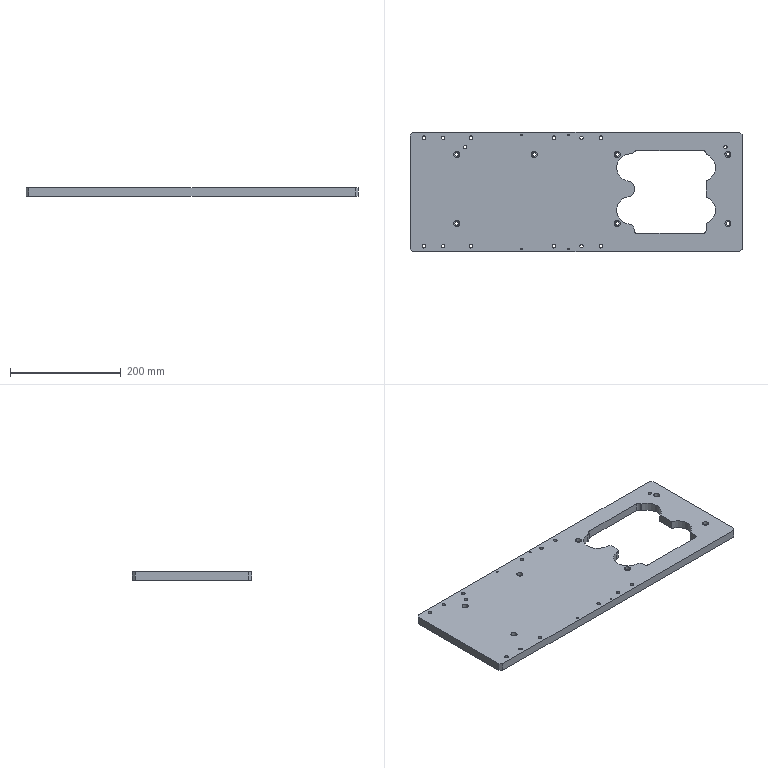CAM job | NX | 3-axis milling, drilling | part box 600 x 216 x 15 mm | stock box 606 x 222 x 16 mm
Tools:
number,name,description,diameter,corner_radius,flute_length,length,flutes
1,D50,Milling Tool-5 Parameters,50.0,0.0,50.0,75.0,2
2,D6A45,Milling Tool-5 Parameters,6.0,0.0,3.0,3.0,2
11,6.6ZT,Drilling Tool,6.6,0.0,35.0,50.0,2
17,5.8ZT,Drilling Tool,5.8,0.0,35.0,50.0,2
16,6.0JD,Milling Tool-5 Parameters,6.0,0.0,30.0,30.0,4
22,3.3ZT,Drilling Tool,3.3,0.0,35.0,50.0,2
8,D6,Milling Tool-5 Parameters,6.0,0.0,50.0,75.0,2
3,D10,Milling Tool-5 Parameters,10.0,0.0,50.0,75.0,2
4,D10JING,Milling Tool-5 Parameters,10.0,0.0,50.0,75.0,2
Operations:
program,operation,operation_type,tool,method,geometry_group,spindle_rpm,surface_speed,feed_per_tooth,feed_cut,feed_plunge,cut_length_mm,path_length_mm,cut_time_min,machine_time_min
1-603-219-15毛胚-AB胶,FLOOR_WALL,VolumeBased25DMillingOperation,D50,METHOD,A,6500.0,1286.0,0.0962,1250.0,100.0,6773.997,6827.997,5.419,5.425
1-603-219-15毛胚-AB胶,DRILLING_COPY_1,Operation,D6A45,METHOD,A,3000.0,56.0,0.0333,200.0,0.0,115.0,1731.497,0.575,0.7366
1-603-219-15毛胚-AB胶,DRILLING_COPY_1_COPY_COPY_1_COPY_1,Operation,6.6ZT,METHOD,A,2000.0,18.0,0.03,120.0,0.0,120.663,1158.62,1.006,1.109
1-603-219-15毛胚-AB胶,DRILLING_COPY_1_COPY_COPY_1_COPY_1_COPY,Operation,6.6ZT,METHOD,A,2000.0,18.0,0.03,120.0,0.0,150.38,1243.952,1.253,1.363
1-603-219-15毛胚-AB胶,DRILLING_COPY_1_COPY_COPY,Operation,5.8ZT,METHOD,A,2000.0,15.0,0.0375,150.0,0.0,127.455,1263.529,0.8497,0.9633
1-603-219-15毛胚-AB胶,DRILLING_COPY_1_COPY_COPY_COPY,Operation,6.0JD,METHOD,A,1000.0,18.0,0.0125,50.0,0.0,111.0,1230.619,2.22,2.332
1-603-219-15毛胚-AB胶,DRILLING_COPY_1_COPY_COPY_COPY_COPY_COPY_COPY_1,Operation,3.3ZT,METHOD,A,2000.0,20.0,0.0375,150.0,0.0,81.966,609.059,0.5464,0.5991
1-603-219-15毛胚-AB胶,ZLEVEL_PROFILE,ZLevelMilling,D10,METHOD,A,7000.0,219.0,0.2143,3000.0,1000.0,24888.547,24959.947,8.328,8.335
1-603-219-15毛胚-AB胶,ZLEVEL_PROFILE_COPY,ZLevelMilling,D10,METHOD,A,7000.0,219.0,0.2143,3000.0,1000.0,9376.422,9448.121,3.157,3.164
1-603-219-15毛胚-AB胶,HOLE_MILLING_1,CylinderMilling,D6,METHOD,A,7000.0,131.0,0.1071,1500.0,100.0,1683.091,3057.075,1.122,1.26
1-603-219-15毛胚-AB胶,ZLEVEL_PROFILE_COPY_COPY_1_COPY_COPY_COPY_1,ZLevelMilling,D6,METHOD,A,7000.0,219.0,0.0714,1000.0,100.0,633.75,723.35,0.6337,0.6427
1-603-219-15毛胚-AB胶,ZLEVEL_PROFILE_COPY_1_COPY_COPY_COPY_COPY_2_COPY,ZLevelMilling,D6A45,METHOD,A,7000.0,131.0,0.0714,1000.0,1000.0,2767.046,9139.675,2.767,3.404
1-603-219-15毛胚-AB胶,ZLEVEL_PROFILE_COPY_1_1,ZLevelMilling,D10JING,METHOD,A,7000.0,219.0,0.0714,1000.0,1000.0,5188.344,5265.094,5.188,5.196